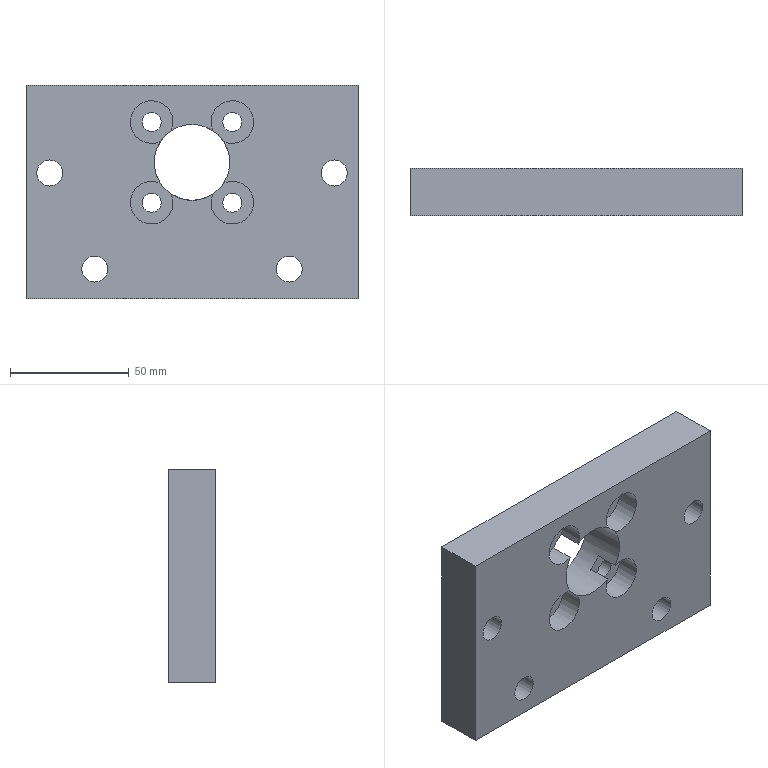Part | NX | features solid 2 | 1 solid | 31 faces | box 140 x 20 x 90 mm | volume 209276 mm3 | cylinder 17 | plane 14 | commonest cylinder face diameters 18 x8 8 x4 11 x4 32 x1
STEP:
#1=CARTESIAN_POINT('',(17.,291.5,-39.));
#2=VERTEX_POINT('',#1);
#3=CARTESIAN_POINT('',(17.,291.5,-35.));
#4=DIRECTION('',(0.,1.,0.));
#5=DIRECTION('',(0.,0.,-1.));
#6=AXIS2_PLACEMENT_3D('',#3,#4,#5);
#7=CIRCLE('',#6,4.);
#8=EDGE_CURVE('',#2,#2,#7,.F.);
#9=ORIENTED_EDGE('',*,*,#8,.T.);
#10=EDGE_LOOP('',(#9));
#11=FACE_BOUND('',#10,.T.);
#12=CARTESIAN_POINT('',(-17.,291.5,-5.));
#13=VERTEX_POINT('',#12);
#14=CARTESIAN_POINT('',(-17.,291.5,-1.));
#15=DIRECTION('',(0.,1.,0.));
#16=DIRECTION('',(0.,0.,-1.));
#17=AXIS2_PLACEMENT_3D('',#14,#15,#16);
#18=CIRCLE('',#17,4.);
#19=EDGE_CURVE('',#13,#13,#18,.F.);
#20=ORIENTED_EDGE('',*,*,#19,.T.);
#21=EDGE_LOOP('',(#20));
#22=FACE_BOUND('',#21,.T.);
#23=CARTESIAN_POINT('',(-70.,291.5,-75.5));
#24=VERTEX_POINT('',#23);
#25=CARTESIAN_POINT('',(-70.,291.5,14.5));
#26=VERTEX_POINT('',#25);
#27=CARTESIAN_POINT('',(-70.,291.5,-75.5));
#28=DIRECTION('',(0.,0.,1.));
#29=VECTOR('',#28,1000.);
#30=LINE('',#27,#29);
#31=EDGE_CURVE('',#24,#26,#30,.T.);
#32=ORIENTED_EDGE('',*,*,#31,.T.);
#33=CARTESIAN_POINT('',(70.,291.5,14.5));
#34=VERTEX_POINT('',#33);
#35=CARTESIAN_POINT('',(0.,291.5,14.5));
#36=DIRECTION('',(-1.,0.,0.));
#37=VECTOR('',#36,1000.);
#38=LINE('',#35,#37);
#39=EDGE_CURVE('',#34,#26,#38,.T.);
#40=ORIENTED_EDGE('',*,*,#39,.F.);
#41=CARTESIAN_POINT('',(70.,291.5,-75.5));
#42=VERTEX_POINT('',#41);
#43=CARTESIAN_POINT('',(70.,291.5,-75.5));
#44=DIRECTION('',(0.,0.,1.));
#45=VECTOR('',#44,1000.);
#46=LINE('',#43,#45);
#47=EDGE_CURVE('',#42,#34,#46,.T.);
#48=ORIENTED_EDGE('',*,*,#47,.F.);
#49=CARTESIAN_POINT('',(0.,291.5,-75.5));
#50=DIRECTION('',(1.,0.,0.));
#51=VECTOR('',#50,1000.);
#52=LINE('',#49,#51);
#53=EDGE_CURVE('',#24,#42,#52,.T.);
#54=ORIENTED_EDGE('',*,*,#53,.F.);
#55=EDGE_LOOP('',(#32,#40,#48,#54));
#56=FACE_BOUND('',#55,.T.);
#57=CARTESIAN_POINT('',(-69.,291.5,-22.5));
#58=VERTEX_POINT('',#57);
#59=CARTESIAN_POINT('',(-60.,291.5,-22.5));
#60=DIRECTION('',(0.,1.,0.));
#61=DIRECTION('',(-1.,0.,0.));
#62=AXIS2_PLACEMENT_3D('',#59,#60,#61);
#63=CIRCLE('',#62,9.);
#64=EDGE_CURVE('',#58,#58,#63,.T.);
#65=ORIENTED_EDGE('',*,*,#64,.F.);
#66=EDGE_LOOP('',(#65));
#67=FACE_BOUND('',#66,.T.);
#68=CARTESIAN_POINT('',(-50.,291.5,-63.));
#69=VERTEX_POINT('',#68);
#70=CARTESIAN_POINT('',(-41.,291.5,-63.));
#71=DIRECTION('',(0.,1.,0.));
#72=DIRECTION('',(-1.,0.,0.));
#73=AXIS2_PLACEMENT_3D('',#70,#71,#72);
#74=CIRCLE('',#73,9.);
#75=EDGE_CURVE('',#69,#69,#74,.T.);
#76=ORIENTED_EDGE('',*,*,#75,.F.);
#77=EDGE_LOOP('',(#76));
#78=FACE_BOUND('',#77,.T.);
#79=CARTESIAN_POINT('',(32.,291.5,-63.));
#80=VERTEX_POINT('',#79);
#81=CARTESIAN_POINT('',(41.,291.5,-63.));
#82=DIRECTION('',(0.,1.,0.));
#83=DIRECTION('',(-1.,0.,0.));
#84=AXIS2_PLACEMENT_3D('',#81,#82,#83);
#85=CIRCLE('',#84,9.);
#86=EDGE_CURVE('',#80,#80,#85,.T.);
#87=ORIENTED_EDGE('',*,*,#86,.F.);
#88=EDGE_LOOP('',(#87));
#89=FACE_BOUND('',#88,.T.);
#90=CARTESIAN_POINT('',(51.,291.5,-22.5));
#91=VERTEX_POINT('',#90);
#92=CARTESIAN_POINT('',(60.,291.5,-22.5));
#93=DIRECTION('',(0.,1.,0.));
#94=DIRECTION('',(-1.,0.,0.));
#95=AXIS2_PLACEMENT_3D('',#92,#93,#94);
#96=CIRCLE('',#95,9.);
#97=EDGE_CURVE('',#91,#91,#96,.T.);
#98=ORIENTED_EDGE('',*,*,#97,.F.);
#99=EDGE_LOOP('',(#98));
#100=FACE_BOUND('',#99,.T.);
#101=CARTESIAN_POINT('',(-17.,291.5,-39.));
#102=VERTEX_POINT('',#101);
#103=CARTESIAN_POINT('',(-17.,291.5,-35.));
#104=DIRECTION('',(0.,1.,0.));
#105=DIRECTION('',(0.,0.,-1.));
#106=AXIS2_PLACEMENT_3D('',#103,#104,#105);
#107=CIRCLE('',#106,4.);
#108=EDGE_CURVE('',#102,#102,#107,.T.);
#109=ORIENTED_EDGE('',*,*,#108,.F.);
#110=EDGE_LOOP('',(#109));
#111=FACE_BOUND('',#110,.T.);
#112=CARTESIAN_POINT('',(17.,291.5,-5.));
#113=VERTEX_POINT('',#112);
#114=CARTESIAN_POINT('',(17.,291.5,-1.));
#115=DIRECTION('',(0.,1.,0.));
#116=DIRECTION('',(0.,0.,-1.));
#117=AXIS2_PLACEMENT_3D('',#114,#115,#116);
#118=CIRCLE('',#117,4.);
#119=EDGE_CURVE('',#113,#113,#118,.T.);
#120=ORIENTED_EDGE('',*,*,#119,.F.);
#121=EDGE_LOOP('',(#120));
#122=FACE_BOUND('',#121,.T.);
#123=CARTESIAN_POINT('',(0.,291.5,-34.));
#124=VERTEX_POINT('',#123);
#125=CARTESIAN_POINT('',(0.,291.5,-18.));
#126=DIRECTION('',(0.,1.,0.));
#127=DIRECTION('',(0.,0.,-1.));
#128=AXIS2_PLACEMENT_3D('',#125,#126,#127);
#129=CIRCLE('',#128,16.);
#130=EDGE_CURVE('',#124,#124,#129,.T.);
#131=ORIENTED_EDGE('',*,*,#130,.F.);
#132=EDGE_LOOP('',(#131));
#133=FACE_BOUND('',#132,.T.);
#134=CARTESIAN_POINT('',(0.,291.5,-75.5));
#135=DIRECTION('',(0.,1.,0.));
#136=DIRECTION('',(0.,0.,1.));
#137=AXIS2_PLACEMENT_3D('',#134,#135,#136);
#138=PLANE('',#137);
#139=ADVANCED_FACE('',(#11,#22,#56,#67,#78,#89,#100,#111,#122,#133),#138,.T.);
#140=CARTESIAN_POINT('',(70.,271.5,-75.5));
#141=VERTEX_POINT('',#140);
#142=CARTESIAN_POINT('',(70.,271.5,14.5));
#143=VERTEX_POINT('',#142);
#144=CARTESIAN_POINT('',(70.,271.5,-75.5));
#145=DIRECTION('',(0.,0.,1.));
#146=VECTOR('',#145,1000.);
#147=LINE('',#144,#146);
#148=EDGE_CURVE('',#141,#143,#147,.T.);
#149=ORIENTED_EDGE('',*,*,#148,.T.);
#150=CARTESIAN_POINT('',(-70.,271.5,14.5));
#151=VERTEX_POINT('',#150);
#152=CARTESIAN_POINT('',(0.,271.5,14.5));
#153=DIRECTION('',(1.,0.,0.));
#154=VECTOR('',#153,1000.);
#155=LINE('',#152,#154);
#156=EDGE_CURVE('',#151,#143,#155,.T.);
#157=ORIENTED_EDGE('',*,*,#156,.F.);
#158=CARTESIAN_POINT('',(-70.,271.5,-75.5));
#159=VERTEX_POINT('',#158);
#160=CARTESIAN_POINT('',(-70.,271.5,-75.5));
#161=DIRECTION('',(0.,0.,-1.));
#162=VECTOR('',#161,1000.);
#163=LINE('',#160,#162);
#164=EDGE_CURVE('',#151,#159,#163,.T.);
#165=ORIENTED_EDGE('',*,*,#164,.T.);
#166=CARTESIAN_POINT('',(0.,271.5,-75.5));
#167=DIRECTION('',(1.,0.,0.));
#168=VECTOR('',#167,1000.);
#169=LINE('',#166,#168);
#170=EDGE_CURVE('',#159,#141,#169,.T.);
#171=ORIENTED_EDGE('',*,*,#170,.T.);
#172=EDGE_LOOP('',(#149,#157,#165,#171));
#173=FACE_BOUND('',#172,.T.);
#174=CARTESIAN_POINT('',(41.,271.5,-68.5));
#175=VERTEX_POINT('',#174);
#176=CARTESIAN_POINT('',(41.,271.5,-63.));
#177=DIRECTION('',(0.,1.,0.));
#178=DIRECTION('',(0.,0.,-1.));
#179=AXIS2_PLACEMENT_3D('',#176,#177,#178);
#180=CIRCLE('',#179,5.5);
#181=EDGE_CURVE('',#175,#175,#180,.T.);
#182=ORIENTED_EDGE('',*,*,#181,.T.);
#183=EDGE_LOOP('',(#182));
#184=FACE_BOUND('',#183,.T.);
#185=CARTESIAN_POINT('',(-41.,271.5,-68.5));
#186=VERTEX_POINT('',#185);
#187=CARTESIAN_POINT('',(-41.,271.5,-63.));
#188=DIRECTION('',(0.,1.,0.));
#189=DIRECTION('',(0.,0.,-1.));
#190=AXIS2_PLACEMENT_3D('',#187,#188,#189);
#191=CIRCLE('',#190,5.5);
#192=EDGE_CURVE('',#186,#186,#191,.T.);
#193=ORIENTED_EDGE('',*,*,#192,.T.);
#194=EDGE_LOOP('',(#193));
#195=FACE_BOUND('',#194,.T.);
#196=CARTESIAN_POINT('',(60.,271.5,-28.));
#197=VERTEX_POINT('',#196);
#198=CARTESIAN_POINT('',(60.,271.5,-22.5));
#199=DIRECTION('',(0.,1.,0.));
#200=DIRECTION('',(0.,0.,-1.));
#201=AXIS2_PLACEMENT_3D('',#198,#199,#200);
#202=CIRCLE('',#201,5.5);
#203=EDGE_CURVE('',#197,#197,#202,.T.);
#204=ORIENTED_EDGE('',*,*,#203,.T.);
#205=EDGE_LOOP('',(#204));
#206=FACE_BOUND('',#205,.T.);
#207=CARTESIAN_POINT('',(-60.,271.5,-28.));
#208=VERTEX_POINT('',#207);
#209=CARTESIAN_POINT('',(-60.,271.5,-22.5));
#210=DIRECTION('',(0.,1.,0.));
#211=DIRECTION('',(0.,0.,-1.));
#212=AXIS2_PLACEMENT_3D('',#209,#210,#211);
#213=CIRCLE('',#212,5.5);
#214=EDGE_CURVE('',#208,#208,#213,.F.);
#215=ORIENTED_EDGE('',*,*,#214,.F.);
#216=EDGE_LOOP('',(#215));
#217=FACE_BOUND('',#216,.T.);
#218=CARTESIAN_POINT('',(-13.392,271.5,-9.245));
#219=VERTEX_POINT('',#218);
#220=CARTESIAN_POINT('',(-13.392,271.5,-26.755));
#221=VERTEX_POINT('',#220);
#222=CARTESIAN_POINT('',(0.,271.5,-18.));
#223=DIRECTION('',(0.,1.,0.));
#224=DIRECTION('',(0.,0.,-1.));
#225=AXIS2_PLACEMENT_3D('',#222,#223,#224);
#226=CIRCLE('',#225,16.);
#227=EDGE_CURVE('',#219,#221,#226,.F.);
#228=ORIENTED_EDGE('',*,*,#227,.F.);
#229=CARTESIAN_POINT('',(-8.755,271.5,-4.608));
#230=VERTEX_POINT('',#229);
#231=CARTESIAN_POINT('',(-17.,271.5,-1.));
#232=DIRECTION('',(0.,1.,0.));
#233=DIRECTION('',(0.,0.,-1.));
#234=AXIS2_PLACEMENT_3D('',#231,#232,#233);
#235=CIRCLE('',#234,9.);
#236=EDGE_CURVE('',#219,#230,#235,.T.);
#237=ORIENTED_EDGE('',*,*,#236,.T.);
#238=CARTESIAN_POINT('',(8.755,271.5,-4.608));
#239=VERTEX_POINT('',#238);
#240=CARTESIAN_POINT('',(0.,271.5,-18.));
#241=DIRECTION('',(0.,1.,0.));
#242=DIRECTION('',(0.,0.,-1.));
#243=AXIS2_PLACEMENT_3D('',#240,#241,#242);
#244=CIRCLE('',#243,16.);
#245=EDGE_CURVE('',#239,#230,#244,.F.);
#246=ORIENTED_EDGE('',*,*,#245,.F.);
#247=CARTESIAN_POINT('',(13.392,271.5,-9.245));
#248=VERTEX_POINT('',#247);
#249=CARTESIAN_POINT('',(17.,271.5,-1.));
#250=DIRECTION('',(0.,1.,0.));
#251=DIRECTION('',(0.,0.,-1.));
#252=AXIS2_PLACEMENT_3D('',#249,#250,#251);
#253=CIRCLE('',#252,9.);
#254=EDGE_CURVE('',#239,#248,#253,.T.);
#255=ORIENTED_EDGE('',*,*,#254,.T.);
#256=CARTESIAN_POINT('',(13.392,271.5,-26.755));
#257=VERTEX_POINT('',#256);
#258=CARTESIAN_POINT('',(0.,271.5,-18.));
#259=DIRECTION('',(0.,1.,0.));
#260=DIRECTION('',(0.,0.,-1.));
#261=AXIS2_PLACEMENT_3D('',#258,#259,#260);
#262=CIRCLE('',#261,16.);
#263=EDGE_CURVE('',#257,#248,#262,.F.);
#264=ORIENTED_EDGE('',*,*,#263,.F.);
#265=CARTESIAN_POINT('',(8.755,271.5,-31.392));
#266=VERTEX_POINT('',#265);
#267=CARTESIAN_POINT('',(17.,271.5,-35.));
#268=DIRECTION('',(0.,1.,0.));
#269=DIRECTION('',(0.,0.,-1.));
#270=AXIS2_PLACEMENT_3D('',#267,#268,#269);
#271=CIRCLE('',#270,9.);
#272=EDGE_CURVE('',#257,#266,#271,.T.);
#273=ORIENTED_EDGE('',*,*,#272,.T.);
#274=CARTESIAN_POINT('',(-8.755,271.5,-31.392));
#275=VERTEX_POINT('',#274);
#276=CARTESIAN_POINT('',(0.,271.5,-18.));
#277=DIRECTION('',(0.,1.,0.));
#278=DIRECTION('',(0.,0.,-1.));
#279=AXIS2_PLACEMENT_3D('',#276,#277,#278);
#280=CIRCLE('',#279,16.);
#281=EDGE_CURVE('',#275,#266,#280,.F.);
#282=ORIENTED_EDGE('',*,*,#281,.F.);
#283=CARTESIAN_POINT('',(-17.,271.5,-35.));
#284=DIRECTION('',(0.,1.,0.));
#285=DIRECTION('',(0.,0.,-1.));
#286=AXIS2_PLACEMENT_3D('',#283,#284,#285);
#287=CIRCLE('',#286,9.);
#288=EDGE_CURVE('',#275,#221,#287,.T.);
#289=ORIENTED_EDGE('',*,*,#288,.T.);
#290=EDGE_LOOP('',(#228,#237,#246,#255,#264,#273,#282,#289));
#291=FACE_BOUND('',#290,.T.);
#292=CARTESIAN_POINT('',(0.,271.5,-75.5));
#293=DIRECTION('',(0.,-1.,0.));
#294=DIRECTION('',(0.,0.,-1.));
#295=AXIS2_PLACEMENT_3D('',#292,#293,#294);
#296=PLANE('',#295);
#297=ADVANCED_FACE('',(#173,#184,#195,#206,#217,#291),#296,.T.);
#298=CARTESIAN_POINT('',(70.,151.5,-75.5));
#299=DIRECTION('',(0.,-1.,0.));
#300=VECTOR('',#299,1000.);
#301=LINE('',#298,#300);
#302=EDGE_CURVE('',#42,#141,#301,.T.);
#303=ORIENTED_EDGE('',*,*,#302,.F.);
#304=ORIENTED_EDGE('',*,*,#47,.T.);
#305=CARTESIAN_POINT('',(70.,291.5,14.5));
#306=DIRECTION('',(0.,1.,0.));
#307=VECTOR('',#306,1000.);
#308=LINE('',#305,#307);
#309=EDGE_CURVE('',#143,#34,#308,.T.);
#310=ORIENTED_EDGE('',*,*,#309,.F.);
#311=ORIENTED_EDGE('',*,*,#148,.F.);
#312=EDGE_LOOP('',(#303,#304,#310,#311));
#313=FACE_BOUND('',#312,.T.);
#314=CARTESIAN_POINT('',(70.,151.5,-75.5));
#315=DIRECTION('',(1.,0.,0.));
#316=DIRECTION('',(0.,0.,-1.));
#317=AXIS2_PLACEMENT_3D('',#314,#315,#316);
#318=PLANE('',#317);
#319=ADVANCED_FACE('',(#313),#318,.T.);
#320=CARTESIAN_POINT('',(-70.,291.5,14.5));
#321=DIRECTION('',(0.,-1.,0.));
#322=VECTOR('',#321,1000.);
#323=LINE('',#320,#322);
#324=EDGE_CURVE('',#26,#151,#323,.T.);
#325=ORIENTED_EDGE('',*,*,#324,.F.);
#326=ORIENTED_EDGE('',*,*,#31,.F.);
#327=CARTESIAN_POINT('',(-70.,151.5,-75.5));
#328=DIRECTION('',(0.,1.,0.));
#329=VECTOR('',#328,1000.);
#330=LINE('',#327,#329);
#331=EDGE_CURVE('',#159,#24,#330,.T.);
#332=ORIENTED_EDGE('',*,*,#331,.F.);
#333=ORIENTED_EDGE('',*,*,#164,.F.);
#334=EDGE_LOOP('',(#325,#326,#332,#333));
#335=FACE_BOUND('',#334,.T.);
#336=CARTESIAN_POINT('',(-70.,151.5,-75.5));
#337=DIRECTION('',(-1.,0.,0.));
#338=DIRECTION('',(0.,0.,1.));
#339=AXIS2_PLACEMENT_3D('',#336,#337,#338);
#340=PLANE('',#339);
#341=ADVANCED_FACE('',(#335),#340,.T.);
#342=ORIENTED_EDGE('',*,*,#331,.T.);
#343=ORIENTED_EDGE('',*,*,#53,.T.);
#344=ORIENTED_EDGE('',*,*,#302,.T.);
#345=ORIENTED_EDGE('',*,*,#170,.F.);
#346=EDGE_LOOP('',(#342,#343,#344,#345));
#347=FACE_BOUND('',#346,.T.);
#348=CARTESIAN_POINT('',(0.,151.5,-75.5));
#349=DIRECTION('',(0.,0.,-1.));
#350=DIRECTION('',(0.,1.,0.));
#351=AXIS2_PLACEMENT_3D('',#348,#349,#350);
#352=PLANE('',#351);
#353=ADVANCED_FACE('',(#347),#352,.T.);
#354=ORIENTED_EDGE('',*,*,#156,.T.);
#355=ORIENTED_EDGE('',*,*,#309,.T.);
#356=ORIENTED_EDGE('',*,*,#39,.T.);
#357=ORIENTED_EDGE('',*,*,#324,.T.);
#358=EDGE_LOOP('',(#354,#355,#356,#357));
#359=FACE_BOUND('',#358,.T.);
#360=CARTESIAN_POINT('',(0.,291.5,14.5));
#361=DIRECTION('',(0.,0.,1.));
#362=DIRECTION('',(0.,-1.,0.));
#363=AXIS2_PLACEMENT_3D('',#360,#361,#362);
#364=PLANE('',#363);
#365=ADVANCED_FACE('',(#359),#364,.T.);
#366=CARTESIAN_POINT('',(60.,280.5,-17.));
#367=VERTEX_POINT('',#366);
#368=CARTESIAN_POINT('',(60.,280.5,-22.5));
#369=DIRECTION('',(0.,1.,0.));
#370=DIRECTION('',(0.,0.,1.));
#371=AXIS2_PLACEMENT_3D('',#368,#369,#370);
#372=CIRCLE('',#371,5.5);
#373=EDGE_CURVE('',#367,#367,#372,.T.);
#374=ORIENTED_EDGE('',*,*,#373,.T.);
#375=EDGE_LOOP('',(#374));
#376=FACE_BOUND('',#375,.T.);
#377=ORIENTED_EDGE('',*,*,#203,.F.);
#378=EDGE_LOOP('',(#377));
#379=FACE_BOUND('',#378,.T.);
#380=CARTESIAN_POINT('',(60.,297.5,-22.5));
#381=DIRECTION('',(0.,1.,0.));
#382=DIRECTION('',(0.,0.,1.));
#383=AXIS2_PLACEMENT_3D('',#380,#381,#382);
#384=CYLINDRICAL_SURFACE('',#383,5.5);
#385=ADVANCED_FACE('',(#376,#379),#384,.F.);
#386=ORIENTED_EDGE('',*,*,#373,.F.);
#387=EDGE_LOOP('',(#386));
#388=FACE_BOUND('',#387,.T.);
#389=CARTESIAN_POINT('',(51.,280.5,-22.5));
#390=VERTEX_POINT('',#389);
#391=CARTESIAN_POINT('',(60.,280.5,-22.5));
#392=DIRECTION('',(0.,-1.,0.));
#393=DIRECTION('',(-1.,0.,0.));
#394=AXIS2_PLACEMENT_3D('',#391,#392,#393);
#395=CIRCLE('',#394,9.);
#396=EDGE_CURVE('',#390,#390,#395,.T.);
#397=ORIENTED_EDGE('',*,*,#396,.F.);
#398=EDGE_LOOP('',(#397));
#399=FACE_BOUND('',#398,.T.);
#400=CARTESIAN_POINT('',(60.,280.5,-22.5));
#401=DIRECTION('',(0.,1.,0.));
#402=DIRECTION('',(0.,0.,1.));
#403=AXIS2_PLACEMENT_3D('',#400,#401,#402);
#404=PLANE('',#403);
#405=ADVANCED_FACE('',(#388,#399),#404,.T.);
#406=CARTESIAN_POINT('',(-60.,280.5,-17.));
#407=VERTEX_POINT('',#406);
#408=CARTESIAN_POINT('',(-60.,280.5,-22.5));
#409=DIRECTION('',(0.,-1.,0.));
#410=DIRECTION('',(0.,0.,1.));
#411=AXIS2_PLACEMENT_3D('',#408,#409,#410);
#412=CIRCLE('',#411,5.5);
#413=EDGE_CURVE('',#407,#407,#412,.T.);
#414=ORIENTED_EDGE('',*,*,#413,.F.);
#415=EDGE_LOOP('',(#414));
#416=FACE_BOUND('',#415,.T.);
#417=ORIENTED_EDGE('',*,*,#214,.T.);
#418=EDGE_LOOP('',(#417));
#419=FACE_BOUND('',#418,.T.);
#420=CARTESIAN_POINT('',(-60.,297.5,-22.5));
#421=DIRECTION('',(0.,1.,0.));
#422=DIRECTION('',(0.,0.,1.));
#423=AXIS2_PLACEMENT_3D('',#420,#421,#422);
#424=CYLINDRICAL_SURFACE('',#423,5.5);
#425=ADVANCED_FACE('',(#416,#419),#424,.F.);
#426=ORIENTED_EDGE('',*,*,#413,.T.);
#427=EDGE_LOOP('',(#426));
#428=FACE_BOUND('',#427,.T.);
#429=CARTESIAN_POINT('',(-69.,280.5,-22.5));
#430=VERTEX_POINT('',#429);
#431=CARTESIAN_POINT('',(-60.,280.5,-22.5));
#432=DIRECTION('',(0.,-1.,0.));
#433=DIRECTION('',(-1.,0.,0.));
#434=AXIS2_PLACEMENT_3D('',#431,#432,#433);
#435=CIRCLE('',#434,9.);
#436=EDGE_CURVE('',#430,#430,#435,.T.);
#437=ORIENTED_EDGE('',*,*,#436,.F.);
#438=EDGE_LOOP('',(#437));
#439=FACE_BOUND('',#438,.T.);
#440=CARTESIAN_POINT('',(-60.,280.5,-22.5));
#441=DIRECTION('',(0.,1.,0.));
#442=DIRECTION('',(0.,0.,1.));
#443=AXIS2_PLACEMENT_3D('',#440,#441,#442);
#444=PLANE('',#443);
#445=ADVANCED_FACE('',(#428,#439),#444,.T.);
#446=CARTESIAN_POINT('',(-41.,280.5,-68.5));
#447=VERTEX_POINT('',#446);
#448=CARTESIAN_POINT('',(-41.,280.5,-63.));
#449=DIRECTION('',(0.,1.,0.));
#450=DIRECTION('',(0.,0.,-1.));
#451=AXIS2_PLACEMENT_3D('',#448,#449,#450);
#452=CIRCLE('',#451,5.5);
#453=EDGE_CURVE('',#447,#447,#452,.F.);
#454=ORIENTED_EDGE('',*,*,#453,.T.);
#455=EDGE_LOOP('',(#454));
#456=FACE_BOUND('',#455,.T.);
#457=CARTESIAN_POINT('',(-50.,280.5,-63.));
#458=VERTEX_POINT('',#457);
#459=CARTESIAN_POINT('',(-41.,280.5,-63.));
#460=DIRECTION('',(0.,-1.,0.));
#461=DIRECTION('',(-1.,0.,0.));
#462=AXIS2_PLACEMENT_3D('',#459,#460,#461);
#463=CIRCLE('',#462,9.);
#464=EDGE_CURVE('',#458,#458,#463,.F.);
#465=ORIENTED_EDGE('',*,*,#464,.T.);
#466=EDGE_LOOP('',(#465));
#467=FACE_BOUND('',#466,.T.);
#468=CARTESIAN_POINT('',(-41.,280.5,-63.));
#469=DIRECTION('',(0.,-1.,0.));
#470=DIRECTION('',(0.,0.,-1.));
#471=AXIS2_PLACEMENT_3D('',#468,#469,#470);
#472=PLANE('',#471);
#473=ADVANCED_FACE('',(#456,#467),#472,.F.);
#474=ORIENTED_EDGE('',*,*,#464,.F.);
#475=EDGE_LOOP('',(#474));
#476=FACE_BOUND('',#475,.T.);
#477=ORIENTED_EDGE('',*,*,#75,.T.);
#478=EDGE_LOOP('',(#477));
#479=FACE_BOUND('',#478,.T.);
#480=CARTESIAN_POINT('',(-41.,291.5,-63.));
#481=DIRECTION('',(0.,-1.,0.));
#482=DIRECTION('',(-1.,0.,0.));
#483=AXIS2_PLACEMENT_3D('',#480,#481,#482);
#484=CYLINDRICAL_SURFACE('',#483,9.);
#485=ADVANCED_FACE('',(#476,#479),#484,.F.);
#486=ORIENTED_EDGE('',*,*,#192,.F.);
#487=EDGE_LOOP('',(#486));
#488=FACE_BOUND('',#487,.T.);
#489=ORIENTED_EDGE('',*,*,#453,.F.);
#490=EDGE_LOOP('',(#489));
#491=FACE_BOUND('',#490,.T.);
#492=CARTESIAN_POINT('',(-41.,296.5,-63.));
#493=DIRECTION('',(0.,-1.,0.));
#494=DIRECTION('',(-1.,0.,0.));
#495=AXIS2_PLACEMENT_3D('',#492,#493,#494);
#496=CYLINDRICAL_SURFACE('',#495,5.5);
#497=ADVANCED_FACE('',(#488,#491),#496,.F.);
#498=CARTESIAN_POINT('',(41.,280.5,-68.5));
#499=VERTEX_POINT('',#498);
#500=CARTESIAN_POINT('',(41.,280.5,-63.));
#501=DIRECTION('',(0.,1.,0.));
#502=DIRECTION('',(0.,0.,-1.));
#503=AXIS2_PLACEMENT_3D('',#500,#501,#502);
#504=CIRCLE('',#503,5.5);
#505=EDGE_CURVE('',#499,#499,#504,.F.);
#506=ORIENTED_EDGE('',*,*,#505,.T.);
#507=EDGE_LOOP('',(#506));
#508=FACE_BOUND('',#507,.T.);
#509=CARTESIAN_POINT('',(32.,280.5,-63.));
#510=VERTEX_POINT('',#509);
#511=CARTESIAN_POINT('',(41.,280.5,-63.));
#512=DIRECTION('',(0.,-1.,0.));
#513=DIRECTION('',(-1.,0.,0.));
#514=AXIS2_PLACEMENT_3D('',#511,#512,#513);
#515=CIRCLE('',#514,9.);
#516=EDGE_CURVE('',#510,#510,#515,.F.);
#517=ORIENTED_EDGE('',*,*,#516,.T.);
#518=EDGE_LOOP('',(#517));
#519=FACE_BOUND('',#518,.T.);
#520=CARTESIAN_POINT('',(41.,280.5,-63.));
#521=DIRECTION('',(0.,-1.,0.));
#522=DIRECTION('',(0.,0.,-1.));
#523=AXIS2_PLACEMENT_3D('',#520,#521,#522);
#524=PLANE('',#523);
#525=ADVANCED_FACE('',(#508,#519),#524,.F.);
#526=ORIENTED_EDGE('',*,*,#516,.F.);
#527=EDGE_LOOP('',(#526));
#528=FACE_BOUND('',#527,.T.);
#529=ORIENTED_EDGE('',*,*,#86,.T.);
#530=EDGE_LOOP('',(#529));
#531=FACE_BOUND('',#530,.T.);
#532=CARTESIAN_POINT('',(41.,291.5,-63.));
#533=DIRECTION('',(0.,-1.,0.));
#534=DIRECTION('',(-1.,0.,0.));
#535=AXIS2_PLACEMENT_3D('',#532,#533,#534);
#536=CYLINDRICAL_SURFACE('',#535,9.);
#537=ADVANCED_FACE('',(#528,#531),#536,.F.);
#538=ORIENTED_EDGE('',*,*,#181,.F.);
#539=EDGE_LOOP('',(#538));
#540=FACE_BOUND('',#539,.T.);
#541=ORIENTED_EDGE('',*,*,#505,.F.);
#542=EDGE_LOOP('',(#541));
#543=FACE_BOUND('',#542,.T.);
#544=CARTESIAN_POINT('',(41.,296.5,-63.));
#545=DIRECTION('',(0.,-1.,0.));
#546=DIRECTION('',(-1.,0.,0.));
#547=AXIS2_PLACEMENT_3D('',#544,#545,#546);
#548=CYLINDRICAL_SURFACE('',#547,5.5);
#549=ADVANCED_FACE('',(#540,#543),#548,.F.);
#550=ORIENTED_EDGE('',*,*,#436,.T.);
#551=EDGE_LOOP('',(#550));
#552=FACE_BOUND('',#551,.T.);
#553=ORIENTED_EDGE('',*,*,#64,.T.);
#554=EDGE_LOOP('',(#553));
#555=FACE_BOUND('',#554,.T.);
#556=CARTESIAN_POINT('',(-60.,291.5,-22.5));
#557=DIRECTION('',(0.,-1.,0.));
#558=DIRECTION('',(-1.,0.,0.));
#559=AXIS2_PLACEMENT_3D('',#556,#557,#558);
#560=CYLINDRICAL_SURFACE('',#559,9.);
#561=ADVANCED_FACE('',(#552,#555),#560,.F.);
#562=ORIENTED_EDGE('',*,*,#396,.T.);
#563=EDGE_LOOP('',(#562));
#564=FACE_BOUND('',#563,.T.);
#565=ORIENTED_EDGE('',*,*,#97,.T.);
#566=EDGE_LOOP('',(#565));
#567=FACE_BOUND('',#566,.T.);
#568=CARTESIAN_POINT('',(60.,291.5,-22.5));
#569=DIRECTION('',(0.,-1.,0.));
#570=DIRECTION('',(-1.,0.,0.));
#571=AXIS2_PLACEMENT_3D('',#568,#569,#570);
#572=CYLINDRICAL_SURFACE('',#571,9.);
#573=ADVANCED_FACE('',(#564,#567),#572,.F.);
#574=CARTESIAN_POINT('',(8.755,281.5,-4.608));
#575=VERTEX_POINT('',#574);
#576=CARTESIAN_POINT('',(8.755,279.,-4.608));
#577=DIRECTION('',(0.,1.,0.));
#578=VECTOR('',#577,1000.);
#579=LINE('',#576,#578);
#580=EDGE_CURVE('',#239,#575,#579,.T.);
#581=ORIENTED_EDGE('',*,*,#580,.T.);
#582=CARTESIAN_POINT('',(13.392,281.5,-9.245));
#583=VERTEX_POINT('',#582);
#584=CARTESIAN_POINT('',(17.,281.5,-1.));
#585=DIRECTION('',(0.,-1.,0.));
#586=DIRECTION('',(0.,0.,-1.));
#587=AXIS2_PLACEMENT_3D('',#584,#585,#586);
#588=CIRCLE('',#587,9.);
#589=EDGE_CURVE('',#583,#575,#588,.T.);
#590=ORIENTED_EDGE('',*,*,#589,.F.);
#591=CARTESIAN_POINT('',(13.392,279.,-9.245));
#592=DIRECTION('',(0.,1.,0.));
#593=VECTOR('',#592,1000.);
#594=LINE('',#591,#593);
#595=EDGE_CURVE('',#583,#248,#594,.F.);
#596=ORIENTED_EDGE('',*,*,#595,.T.);
#597=ORIENTED_EDGE('',*,*,#254,.F.);
#598=EDGE_LOOP('',(#581,#590,#596,#597));
#599=FACE_BOUND('',#598,.T.);
#600=CARTESIAN_POINT('',(17.,271.5,-1.));
#601=DIRECTION('',(0.,1.,0.));
#602=DIRECTION('',(-1.,0.,0.));
#603=AXIS2_PLACEMENT_3D('',#600,#601,#602);
#604=CYLINDRICAL_SURFACE('',#603,9.);
#605=ADVANCED_FACE('',(#599),#604,.F.);
#606=ORIENTED_EDGE('',*,*,#272,.F.);
#607=CARTESIAN_POINT('',(13.392,281.5,-26.755));
#608=VERTEX_POINT('',#607);
#609=CARTESIAN_POINT('',(13.392,279.,-26.755));
#610=DIRECTION('',(0.,1.,0.));
#611=VECTOR('',#610,1000.);
#612=LINE('',#609,#611);
#613=EDGE_CURVE('',#608,#257,#612,.F.);
#614=ORIENTED_EDGE('',*,*,#613,.F.);
#615=CARTESIAN_POINT('',(8.755,281.5,-31.392));
#616=VERTEX_POINT('',#615);
#617=CARTESIAN_POINT('',(17.,281.5,-35.));
#618=DIRECTION('',(0.,-1.,0.));
#619=DIRECTION('',(0.,0.,-1.));
#620=AXIS2_PLACEMENT_3D('',#617,#618,#619);
#621=CIRCLE('',#620,9.);
#622=EDGE_CURVE('',#616,#608,#621,.T.);
#623=ORIENTED_EDGE('',*,*,#622,.F.);
#624=CARTESIAN_POINT('',(8.755,279.,-31.392));
#625=DIRECTION('',(0.,1.,0.));
#626=VECTOR('',#625,1000.);
#627=LINE('',#624,#626);
#628=EDGE_CURVE('',#266,#616,#627,.T.);
#629=ORIENTED_EDGE('',*,*,#628,.F.);
#630=EDGE_LOOP('',(#606,#614,#623,#629));
#631=FACE_BOUND('',#630,.T.);
#632=CARTESIAN_POINT('',(17.,271.5,-35.));
#633=DIRECTION('',(0.,1.,0.));
#634=DIRECTION('',(-1.,0.,0.));
#635=AXIS2_PLACEMENT_3D('',#632,#633,#634);
#636=CYLINDRICAL_SURFACE('',#635,9.);
#637=ADVANCED_FACE('',(#631),#636,.F.);
#638=CARTESIAN_POINT('',(-13.392,281.5,-9.245));
#639=VERTEX_POINT('',#638);
#640=CARTESIAN_POINT('',(-13.392,279.,-9.245));
#641=DIRECTION('',(0.,1.,0.));
#642=VECTOR('',#641,1000.);
#643=LINE('',#640,#642);
#644=EDGE_CURVE('',#639,#219,#643,.F.);
#645=ORIENTED_EDGE('',*,*,#644,.F.);
#646=CARTESIAN_POINT('',(-8.755,281.5,-4.608));
#647=VERTEX_POINT('',#646);
#648=CARTESIAN_POINT('',(-17.,281.5,-1.));
#649=DIRECTION('',(0.,-1.,0.));
#650=DIRECTION('',(0.,0.,-1.));
#651=AXIS2_PLACEMENT_3D('',#648,#649,#650);
#652=CIRCLE('',#651,9.);
#653=EDGE_CURVE('',#647,#639,#652,.T.);
#654=ORIENTED_EDGE('',*,*,#653,.F.);
#655=CARTESIAN_POINT('',(-8.755,279.,-4.608));
#656=DIRECTION('',(0.,1.,0.));
#657=VECTOR('',#656,1000.);
#658=LINE('',#655,#657);
#659=EDGE_CURVE('',#230,#647,#658,.T.);
#660=ORIENTED_EDGE('',*,*,#659,.F.);
#661=ORIENTED_EDGE('',*,*,#236,.F.);
#662=EDGE_LOOP('',(#645,#654,#660,#661));
#663=FACE_BOUND('',#662,.T.);
#664=CARTESIAN_POINT('',(-17.,271.5,-1.));
#665=DIRECTION('',(0.,1.,0.));
#666=DIRECTION('',(-1.,0.,0.));
#667=AXIS2_PLACEMENT_3D('',#664,#665,#666);
#668=CYLINDRICAL_SURFACE('',#667,9.);
#669=ADVANCED_FACE('',(#663),#668,.F.);
#670=CARTESIAN_POINT('',(-8.755,281.5,-31.392));
#671=VERTEX_POINT('',#670);
#672=CARTESIAN_POINT('',(-8.755,279.,-31.392));
#673=DIRECTION('',(0.,1.,0.));
#674=VECTOR('',#673,1000.);
#675=LINE('',#672,#674);
#676=EDGE_CURVE('',#275,#671,#675,.T.);
#677=ORIENTED_EDGE('',*,*,#676,.T.);
#678=CARTESIAN_POINT('',(-13.392,281.5,-26.755));
#679=VERTEX_POINT('',#678);
#680=CARTESIAN_POINT('',(-17.,281.5,-35.));
#681=DIRECTION('',(0.,-1.,0.));
#682=DIRECTION('',(0.,0.,-1.));
#683=AXIS2_PLACEMENT_3D('',#680,#681,#682);
#684=CIRCLE('',#683,9.);
#685=EDGE_CURVE('',#679,#671,#684,.T.);
#686=ORIENTED_EDGE('',*,*,#685,.F.);
#687=CARTESIAN_POINT('',(-13.392,279.,-26.755));
#688=DIRECTION('',(0.,1.,0.));
#689=VECTOR('',#688,1000.);
#690=LINE('',#687,#689);
#691=EDGE_CURVE('',#679,#221,#690,.F.);
#692=ORIENTED_EDGE('',*,*,#691,.T.);
#693=ORIENTED_EDGE('',*,*,#288,.F.);
#694=EDGE_LOOP('',(#677,#686,#692,#693));
#695=FACE_BOUND('',#694,.T.);
#696=CARTESIAN_POINT('',(-17.,271.5,-35.));
#697=DIRECTION('',(0.,1.,0.));
#698=DIRECTION('',(-1.,0.,0.));
#699=AXIS2_PLACEMENT_3D('',#696,#697,#698);
#700=CYLINDRICAL_SURFACE('',#699,9.);
#701=ADVANCED_FACE('',(#695),#700,.F.);
#702=ORIENTED_EDGE('',*,*,#130,.T.);
#703=EDGE_LOOP('',(#702));
#704=FACE_BOUND('',#703,.T.);
#705=ORIENTED_EDGE('',*,*,#628,.T.);
#706=CARTESIAN_POINT('',(0.,281.5,-18.));
#707=DIRECTION('',(0.,-1.,0.));
#708=DIRECTION('',(0.,0.,-1.));
#709=AXIS2_PLACEMENT_3D('',#706,#707,#708);
#710=CIRCLE('',#709,16.);
#711=EDGE_CURVE('',#616,#608,#710,.T.);
#712=ORIENTED_EDGE('',*,*,#711,.T.);
#713=ORIENTED_EDGE('',*,*,#613,.T.);
#714=ORIENTED_EDGE('',*,*,#263,.T.);
#715=ORIENTED_EDGE('',*,*,#595,.F.);
#716=CARTESIAN_POINT('',(0.,281.5,-18.));
#717=DIRECTION('',(0.,-1.,0.));
#718=DIRECTION('',(0.,0.,-1.));
#719=AXIS2_PLACEMENT_3D('',#716,#717,#718);
#720=CIRCLE('',#719,16.);
#721=EDGE_CURVE('',#583,#575,#720,.T.);
#722=ORIENTED_EDGE('',*,*,#721,.T.);
#723=ORIENTED_EDGE('',*,*,#580,.F.);
#724=ORIENTED_EDGE('',*,*,#245,.T.);
#725=ORIENTED_EDGE('',*,*,#659,.T.);
#726=CARTESIAN_POINT('',(0.,281.5,-18.));
#727=DIRECTION('',(0.,-1.,0.));
#728=DIRECTION('',(0.,0.,-1.));
#729=AXIS2_PLACEMENT_3D('',#726,#727,#728);
#730=CIRCLE('',#729,16.);
#731=EDGE_CURVE('',#639,#647,#730,.F.);
#732=ORIENTED_EDGE('',*,*,#731,.F.);
#733=ORIENTED_EDGE('',*,*,#644,.T.);
#734=ORIENTED_EDGE('',*,*,#227,.T.);
#735=ORIENTED_EDGE('',*,*,#691,.F.);
#736=CARTESIAN_POINT('',(0.,281.5,-18.));
#737=DIRECTION('',(0.,-1.,0.));
#738=DIRECTION('',(0.,0.,-1.));
#739=AXIS2_PLACEMENT_3D('',#736,#737,#738);
#740=CIRCLE('',#739,16.);
#741=EDGE_CURVE('',#679,#671,#740,.T.);
#742=ORIENTED_EDGE('',*,*,#741,.T.);
#743=ORIENTED_EDGE('',*,*,#676,.F.);
#744=ORIENTED_EDGE('',*,*,#281,.T.);
#745=EDGE_LOOP('',(#705,#712,#713,#714,#715,#722,#723,#724,#725,#732,#733,#734,#735,#742,#743,#744));
#746=FACE_BOUND('',#745,.T.);
#747=CARTESIAN_POINT('',(0.,257.5,-18.));
#748=DIRECTION('',(0.,1.,0.));
#749=DIRECTION('',(0.,0.,1.));
#750=AXIS2_PLACEMENT_3D('',#747,#748,#749);
#751=CYLINDRICAL_SURFACE('',#750,16.);
#752=ADVANCED_FACE('',(#704,#746),#751,.F.);
#753=ORIENTED_EDGE('',*,*,#721,.F.);
#754=ORIENTED_EDGE('',*,*,#589,.T.);
#755=EDGE_LOOP('',(#753,#754));
#756=FACE_BOUND('',#755,.T.);
#757=CARTESIAN_POINT('',(17.,281.5,-5.));
#758=VERTEX_POINT('',#757);
#759=CARTESIAN_POINT('',(17.,281.5,-1.));
#760=DIRECTION('',(0.,-1.,0.));
#761=DIRECTION('',(0.,0.,-1.));
#762=AXIS2_PLACEMENT_3D('',#759,#760,#761);
#763=CIRCLE('',#762,4.);
#764=EDGE_CURVE('',#758,#758,#763,.T.);
#765=ORIENTED_EDGE('',*,*,#764,.F.);
#766=EDGE_LOOP('',(#765));
#767=FACE_BOUND('',#766,.T.);
#768=CARTESIAN_POINT('',(17.,281.5,-1.));
#769=DIRECTION('',(0.,-1.,0.));
#770=DIRECTION('',(0.,0.,1.));
#771=AXIS2_PLACEMENT_3D('',#768,#769,#770);
#772=PLANE('',#771);
#773=ADVANCED_FACE('',(#756,#767),#772,.T.);
#774=ORIENTED_EDGE('',*,*,#711,.F.);
#775=ORIENTED_EDGE('',*,*,#622,.T.);
#776=EDGE_LOOP('',(#774,#775));
#777=FACE_BOUND('',#776,.T.);
#778=CARTESIAN_POINT('',(17.,281.5,-39.));
#779=VERTEX_POINT('',#778);
#780=CARTESIAN_POINT('',(17.,281.5,-35.));
#781=DIRECTION('',(0.,-1.,0.));
#782=DIRECTION('',(0.,0.,-1.));
#783=AXIS2_PLACEMENT_3D('',#780,#781,#782);
#784=CIRCLE('',#783,4.);
#785=EDGE_CURVE('',#779,#779,#784,.T.);
#786=ORIENTED_EDGE('',*,*,#785,.F.);
#787=EDGE_LOOP('',(#786));
#788=FACE_BOUND('',#787,.T.);
#789=CARTESIAN_POINT('',(17.,281.5,-35.));
#790=DIRECTION('',(0.,-1.,0.));
#791=DIRECTION('',(0.,0.,1.));
#792=AXIS2_PLACEMENT_3D('',#789,#790,#791);
#793=PLANE('',#792);
#794=ADVANCED_FACE('',(#777,#788),#793,.T.);
#795=ORIENTED_EDGE('',*,*,#119,.T.);
#796=EDGE_LOOP('',(#795));
#797=FACE_BOUND('',#796,.T.);
#798=ORIENTED_EDGE('',*,*,#764,.T.);
#799=EDGE_LOOP('',(#798));
#800=FACE_BOUND('',#799,.T.);
#801=CARTESIAN_POINT('',(17.,286.5,-1.));
#802=DIRECTION('',(0.,-1.,0.));
#803=DIRECTION('',(0.,0.,1.));
#804=AXIS2_PLACEMENT_3D('',#801,#802,#803);
#805=CYLINDRICAL_SURFACE('',#804,4.);
#806=ADVANCED_FACE('',(#797,#800),#805,.F.);
#807=ORIENTED_EDGE('',*,*,#741,.F.);
#808=ORIENTED_EDGE('',*,*,#685,.T.);
#809=EDGE_LOOP('',(#807,#808));
#810=FACE_BOUND('',#809,.T.);
#811=CARTESIAN_POINT('',(-17.,281.5,-39.));
#812=VERTEX_POINT('',#811);
#813=CARTESIAN_POINT('',(-17.,281.5,-35.));
#814=DIRECTION('',(0.,-1.,0.));
#815=DIRECTION('',(0.,0.,-1.));
#816=AXIS2_PLACEMENT_3D('',#813,#814,#815);
#817=CIRCLE('',#816,4.);
#818=EDGE_CURVE('',#812,#812,#817,.T.);
#819=ORIENTED_EDGE('',*,*,#818,.F.);
#820=EDGE_LOOP('',(#819));
#821=FACE_BOUND('',#820,.T.);
#822=CARTESIAN_POINT('',(-17.,281.5,-35.));
#823=DIRECTION('',(0.,-1.,0.));
#824=DIRECTION('',(0.,0.,1.));
#825=AXIS2_PLACEMENT_3D('',#822,#823,#824);
#826=PLANE('',#825);
#827=ADVANCED_FACE('',(#810,#821),#826,.T.);
#828=CARTESIAN_POINT('',(-17.,281.5,-5.));
#829=VERTEX_POINT('',#828);
#830=CARTESIAN_POINT('',(-17.,281.5,-1.));
#831=DIRECTION('',(0.,-1.,0.));
#832=DIRECTION('',(0.,0.,-1.));
#833=AXIS2_PLACEMENT_3D('',#830,#831,#832);
#834=CIRCLE('',#833,4.);
#835=EDGE_CURVE('',#829,#829,#834,.T.);
#836=ORIENTED_EDGE('',*,*,#835,.F.);
#837=EDGE_LOOP('',(#836));
#838=FACE_BOUND('',#837,.T.);
#839=ORIENTED_EDGE('',*,*,#653,.T.);
#840=ORIENTED_EDGE('',*,*,#731,.T.);
#841=EDGE_LOOP('',(#839,#840));
#842=FACE_BOUND('',#841,.T.);
#843=CARTESIAN_POINT('',(-17.,281.5,-1.));
#844=DIRECTION('',(0.,-1.,0.));
#845=DIRECTION('',(0.,0.,1.));
#846=AXIS2_PLACEMENT_3D('',#843,#844,#845);
#847=PLANE('',#846);
#848=ADVANCED_FACE('',(#838,#842),#847,.T.);
#849=ORIENTED_EDGE('',*,*,#108,.T.);
#850=EDGE_LOOP('',(#849));
#851=FACE_BOUND('',#850,.T.);
#852=ORIENTED_EDGE('',*,*,#818,.T.);
#853=EDGE_LOOP('',(#852));
#854=FACE_BOUND('',#853,.T.);
#855=CARTESIAN_POINT('',(-17.,286.5,-35.));
#856=DIRECTION('',(0.,-1.,0.));
#857=DIRECTION('',(0.,0.,1.));
#858=AXIS2_PLACEMENT_3D('',#855,#856,#857);
#859=CYLINDRICAL_SURFACE('',#858,4.);
#860=ADVANCED_FACE('',(#851,#854),#859,.F.);
#861=ORIENTED_EDGE('',*,*,#19,.F.);
#862=EDGE_LOOP('',(#861));
#863=FACE_BOUND('',#862,.T.);
#864=ORIENTED_EDGE('',*,*,#835,.T.);
#865=EDGE_LOOP('',(#864));
#866=FACE_BOUND('',#865,.T.);
#867=CARTESIAN_POINT('',(-17.,286.5,-1.));
#868=DIRECTION('',(0.,-1.,0.));
#869=DIRECTION('',(0.,0.,1.));
#870=AXIS2_PLACEMENT_3D('',#867,#868,#869);
#871=CYLINDRICAL_SURFACE('',#870,4.);
#872=ADVANCED_FACE('',(#863,#866),#871,.F.);
#873=ORIENTED_EDGE('',*,*,#8,.F.);
#874=EDGE_LOOP('',(#873));
#875=FACE_BOUND('',#874,.T.);
#876=ORIENTED_EDGE('',*,*,#785,.T.);
#877=EDGE_LOOP('',(#876));
#878=FACE_BOUND('',#877,.T.);
#879=CARTESIAN_POINT('',(17.,286.5,-35.));
#880=DIRECTION('',(0.,-1.,0.));
#881=DIRECTION('',(0.,0.,1.));
#882=AXIS2_PLACEMENT_3D('',#879,#880,#881);
#883=CYLINDRICAL_SURFACE('',#882,4.);
#884=ADVANCED_FACE('',(#875,#878),#883,.F.);
#885=CLOSED_SHELL('',(#139,#297,#319,#341,#353,#365,#385,#405,#425,#445,#473,#485,#497,#525,#537,#549,#561,#573,#605,#637,#669,#701,#752,#773,#794,#806,#827,#848,#860,#872,#884));
#886=MANIFOLD_SOLID_BREP('',#885);
#887=(LENGTH_UNIT()NAMED_UNIT(*)SI_UNIT(.MILLI.,.METRE.));
#888=UNCERTAINTY_MEASURE_WITH_UNIT(LENGTH_MEASURE(0.00001),#887,'','');
#889=(NAMED_UNIT(*)PLANE_ANGLE_UNIT()SI_UNIT($,.RADIAN.));
#890=(NAMED_UNIT(*)SI_UNIT($,.STERADIAN.)SOLID_ANGLE_UNIT());
#891=(GEOMETRIC_REPRESENTATION_CONTEXT(3)GLOBAL_UNCERTAINTY_ASSIGNED_CONTEXT((#888))GLOBAL_UNIT_ASSIGNED_CONTEXT((#887,#889,#890))REPRESENTATION_CONTEXT('',''));
#892=ADVANCED_BREP_SHAPE_REPRESENTATION('',(#886),#891);